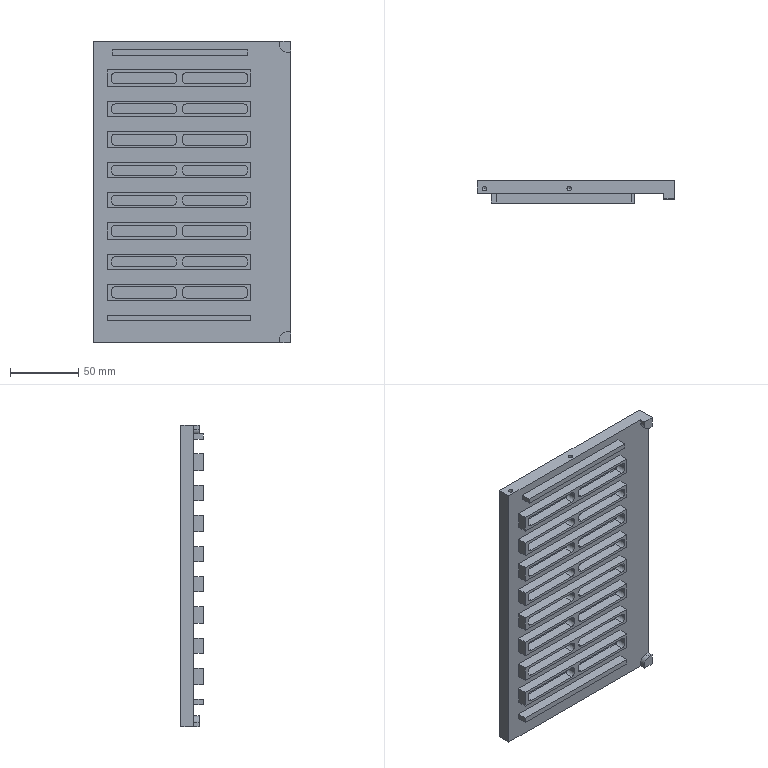NC program | NX | posted with a generic post | part box 144.5 x 16.5 x 221 mm
Lines 3378 to 4181 of 8751:
(动态加工0.5_COPY_1 , TOOL : D5-15-D6-50-3T-ROUGH)
N6748 T03 M6
N6750 G53
N6752 G17 G0 G90 X22.619 Y-60.332 B0. C0. S5000 M3
N6754 G43 Z20. H3
N6756 Z-4.299
N6758 G94 G1 X22.636 Y-60.481 Z-5.236 F1500.
N6760 X22.653 Y-60.63 Z-5.607
N6762 X22.67 Y-60.779 Z-5.879
N6764 X22.686 Y-60.928 Z-6.099
N6766 X22.703 Y-61.077 Z-6.283
N6768 X22.72 Y-61.226 Z-6.441
N6770 X22.737 Y-61.375 Z-6.579
N6772 X22.754 Y-61.524 Z-6.699
N6774 X22.771 Y-61.673 Z-6.804
N6776 X22.787 Y-61.822 Z-6.897
N6778 X22.804 Y-61.971 Z-6.978
N6780 X22.821 Y-62.121 Z-7.049
N6782 X22.838 Y-62.27 Z-7.109
N6784 X22.855 Y-62.419 Z-7.161
N6786 X22.872 Y-62.568 Z-7.204
N6788 X22.888 Y-62.717 Z-7.238
N6790 X22.905 Y-62.866 Z-7.265
N6792 X22.922 Y-63.015 Z-7.284
N6794 X22.939 Y-63.164 Z-7.295
N6796 X22.956 Y-63.313 Z-7.299
N6798 X23.045 Y-64.102
N6800 G3 X23.547 Y-64.55 R0.505
N6802 X25.298 Y-63.147 R2.001
N6804 G1 X25.3 Y-62.787
N6806 G2 X24.701 Y-64.149 R1.509
N6808 X23.619 Y-64.55 R1.349
N6810 G3 X25.295 Y-63.519 R1.549
N6812 G1 X25.3 Y-63.159
N6814 G2 X24.653 Y-64.395 R1.23
N6816 X24.029 Y-64.55 R0.89
N6818 G3 X25.296 Y-63.769 R1.137
N6820 G1 X25.3 Y-63.5
N6822 G2 X24.356 Y-64.55 R0.926
N6824 G3 X25.3 Y-63.914 R0.806
N6826 G1 Y-63.757
N6828 G2 X24.582 Y-64.55 R0.691
N6830 G3 X25.3 Y-63.918 R0.603
N6832 G2 X25.238 Y-64.239 R0.648
N6834 X24.828 Y-64.537 R0.53
N6836 X24.281 Y-64.188 R0.506
N6838 G1 X24.007 Y-63.313
N6840 X23.962 Y-63.17 Z-7.295
N6842 X23.917 Y-63.027 Z-7.284
N6844 X23.872 Y-62.884 Z-7.265
N6846 X23.827 Y-62.741 Z-7.238
N6848 X23.782 Y-62.598 Z-7.204
N6850 X23.737 Y-62.454 Z-7.161
N6852 X23.692 Y-62.311 Z-7.109
N6854 X23.647 Y-62.168 Z-7.049
N6856 X23.602 Y-62.025 Z-6.978
N6858 X23.557 Y-61.882 Z-6.897
N6860 X23.512 Y-61.739 Z-6.804
N6862 X23.467 Y-61.596 Z-6.699
N6864 X23.422 Y-61.453 Z-6.579
N6866 X23.377 Y-61.31 Z-6.441
N6868 X23.332 Y-61.166 Z-6.283
N6870 X23.288 Y-61.023 Z-6.099
N6872 X23.243 Y-60.88 Z-5.879
N6874 X23.198 Y-60.737 Z-5.607
N6876 X23.153 Y-60.594 Z-5.236
N6878 X23.108 Y-60.451 Z-4.299
N6880 G0 Z20.
N6882 X-21.064 Y-62.355
N6884 Z-4.299
N6886 G1 X-21.214 Y-62.353 Z-5.236
N6888 X-21.364 Y-62.35 Z-5.607
N6890 X-21.514 Y-62.347 Z-5.879
N6892 X-21.664 Y-62.345 Z-6.099
N6894 X-21.814 Y-62.342 Z-6.283
N6896 X-21.964 Y-62.34 Z-6.441
N6898 X-22.114 Y-62.337 Z-6.579
N6900 X-22.264 Y-62.335 Z-6.699
N6902 X-22.413 Y-62.332 Z-6.804
N6904 X-22.563 Y-62.33 Z-6.897
N6906 X-22.713 Y-62.327 Z-6.978
N6908 X-22.863 Y-62.324 Z-7.049
N6910 X-23.013 Y-62.322 Z-7.109
N6912 X-23.163 Y-62.319 Z-7.161
N6914 X-23.313 Y-62.317 Z-7.204
N6916 X-23.463 Y-62.314 Z-7.238
N6918 X-23.613 Y-62.312 Z-7.265
N6920 X-23.763 Y-62.309 Z-7.284
N6922 X-23.913 Y-62.307 Z-7.295
N6924 X-24.063 Y-62.304 Z-7.299
N6926 X-24.786 Y-62.292
N6928 G3 X-25.3 Y-62.797 R0.505
N6930 X-23.903 Y-64.548 R2.01
N6932 G1 X-23.541 Y-64.55
N6934 G2 X-24.913 Y-63.935 R1.515
N6936 X-25.3 Y-62.885 R1.328
N6938 G3 X-24.256 Y-64.547 R1.526
N6940 G1 X-23.905 Y-64.55
N6942 G2 X-25.144 Y-63.904 R1.23
N6944 X-25.3 Y-63.278 R0.893
N6946 G3 X-24.532 Y-64.545 R1.143
N6948 G1 X-24.259 Y-64.55
N6950 G2 X-25.3 Y-63.607 R0.924
N6952 G3 X-24.668 Y-64.55 R0.807
N6954 G1 X-24.488
N6956 G2 X-25.3 Y-63.854 R0.694
N6958 G3 X-24.69 Y-64.55 R0.594
N6960 G2 X-24.988 Y-64.488 R0.633
N6962 X-25.287 Y-64.078 R0.53
N6964 X-24.955 Y-63.534 R0.506
N6966 G1 X-24.063 Y-63.221
N6968 X-23.922 Y-63.171 Z-7.295
N6970 X-23.78 Y-63.121 Z-7.284
N6972 X-23.639 Y-63.071 Z-7.265
N6974 X-23.497 Y-63.021 Z-7.238
N6976 X-23.356 Y-62.972 Z-7.204
N6978 X-23.214 Y-62.922 Z-7.161
N6980 X-23.073 Y-62.872 Z-7.109
N6982 X-22.931 Y-62.822 Z-7.049
N6984 X-22.79 Y-62.772 Z-6.978
N6986 X-22.648 Y-62.723 Z-6.897
N6988 X-22.507 Y-62.673 Z-6.804
N6990 X-22.365 Y-62.623 Z-6.699
N6992 X-22.224 Y-62.573 Z-6.579
N6994 X-22.082 Y-62.524 Z-6.441
N6996 X-21.941 Y-62.474 Z-6.283
N6998 X-21.799 Y-62.424 Z-6.099
N7000 X-21.658 Y-62.374 Z-5.879
N7002 X-21.516 Y-62.324 Z-5.607
N7004 X-21.375 Y-62.275 Z-5.236
N7006 X-21.233 Y-62.225 Z-4.299
N7008 G0 Z20.
N7010 X-21.434 Y-61.7
N7012 Z0.3
N7014 G1 X-21.565 Y-61.773 Z-0.637
N7016 X-21.697 Y-61.845 Z-1.008
N7018 X-21.828 Y-61.917 Z-1.28
N7020 X-21.96 Y-61.989 Z-1.5
N7022 X-22.091 Y-62.062 Z-1.684
N7024 X-22.223 Y-62.134 Z-1.842
N7026 X-22.354 Y-62.206 Z-1.98
N7028 X-22.486 Y-62.278 Z-2.1
N7030 X-22.617 Y-62.351 Z-2.205
N7032 X-22.749 Y-62.423 Z-2.298
N7034 X-22.88 Y-62.495 Z-2.379
N7036 X-23.012 Y-62.567 Z-2.45
N7038 X-23.143 Y-62.64 Z-2.51
N7040 X-23.274 Y-62.712 Z-2.562
N7042 X-23.406 Y-62.784 Z-2.605
N7044 X-23.537 Y-62.856 Z-2.639
N7046 X-23.669 Y-62.928 Z-2.666
N7048 X-23.8 Y-63.001 Z-2.685
N7050 X-23.932 Y-63.073 Z-2.696
N7052 X-24.063 Y-63.145 Z-2.7
N7054 X-24.908 Y-63.609
N7056 G3 X-24.845 Y-64.524 R0.505
N7058 X-23.74 Y-64.767 R4.988
N7060 G1 X24.383 Y-64.764
N7062 G3 X25.245 Y-64.348 R1.003
N7064 G1 X25.284 Y-64.243
N7066 G3 X24.637 Y-63.617 R0.519
N7068 G1 X24.364 Y-63.694
N7070 X24.094 Y-63.781
N7072 G3 X24.32 Y-64.767 R0.519
N7074 X25.173 Y-64.536 R1.052
N7076 X25.3 Y-64.178 R0.693
N7078 G2 X24.644 Y-64.767 R0.579
N7080 G3 X24.992 Y-64.703 R0.692
N7082 X25.237 Y-64.457 R0.561
N7084 X25.076 Y-63.864 R0.501
N7086 G1 X24.869 Y-63.709
N7088 X24.486 Y-63.417 Z-2.603
N7090 X24.095 Y-63.137 Z-2.505
N7092 X24.071 Y-63.125 Z-2.5
N7094 X23.967 Y-63.093 F15000.
N7096 X23.86 Y-63.08
N7098 X-22.363 Y-63.39
N7100 G3 X-22.698 Y-63.521 R0.509
N7102 G1 X-22.818 Y-63.679 Z-2.54 F1500.
N7104 X-22.916 Y-63.85 Z-2.58
N7106 X-23.216 Y-64.362 Z-2.7
N7108 X-23.306 Y-64.516
N7110 X-23.421 Y-64.652
N7112 G2 X-23.74 Y-64.767 R0.511
N7114 X-25.032 Y-64.527 R2.277
N7116 X-25.25 Y-64.288 R0.996
N7118 X-24.624 Y-63.524 R0.55
N7120 G1 X-24.244 Y-63.611
N7122 X-23.868 Y-63.709
N7124 G2 X-24.078 Y-64.767 R0.55
N7126 X-25.147 Y-64.489 R1.427
N7128 X-25.287 Y-64.236 R1.13
N7130 X-24.597 Y-63.63 R0.522
N7132 G1 X-24.179 Y-63.792
N7134 G2 X-24.438 Y-64.767 R0.522
N7136 X-25.293 Y-64.257 R0.747
N7138 G1 X-25.3 Y-64.178
N7140 G3 X-24.599 Y-64.767 R0.59
N7142 G2 X-25.031 Y-64.687 R0.792
N7144 X-25.237 Y-64.457 R0.524
N7146 X-24.917 Y-63.779 R0.505
N7148 G1 X-24.063 Y-63.521
N7150 X-23.92 Y-63.477 Z-2.696
N7152 X-23.776 Y-63.434 Z-2.685
N7154 X-23.633 Y-63.39 Z-2.666
N7156 X-23.489 Y-63.347 Z-2.639
N7158 X-23.345 Y-63.304 Z-2.605
N7160 X-23.202 Y-63.26 Z-2.562
N7162 X-23.058 Y-63.217 Z-2.51
N7164 X-22.915 Y-63.173 Z-2.45
N7166 X-22.771 Y-63.13 Z-2.379
N7168 X-22.627 Y-63.087 Z-2.298
N7170 X-22.484 Y-63.043 Z-2.205
N7172 X-22.34 Y-63. Z-2.1
N7174 X-22.197 Y-62.956 Z-1.98
N7176 X-22.053 Y-62.913 Z-1.842
N7178 X-21.91 Y-62.87 Z-1.684
N7180 X-21.766 Y-62.826 Z-1.5
N7182 X-21.622 Y-62.783 Z-1.28
N7184 X-21.479 Y-62.739 Z-1.008
N7186 X-21.335 Y-62.696 Z-0.637
N7188 X-21.192 Y-62.652 Z0.3
N7190 G0 Z20.
N7192 X-21.369 Y-62.09
N7194 Z0.6
N7196 G1 X-21.504 Y-62.156 Z-0.337
N7198 X-21.639 Y-62.222 Z-0.708
N7200 X-21.773 Y-62.288 Z-0.98
N7202 X-21.908 Y-62.354 Z-1.2
N7204 X-22.043 Y-62.42 Z-1.384
N7206 X-22.177 Y-62.486 Z-1.542
N7208 X-22.312 Y-62.552 Z-1.68
N7210 X-22.447 Y-62.618 Z-1.8
N7212 X-22.582 Y-62.684 Z-1.905
N7214 X-22.716 Y-62.75 Z-1.998
N7216 X-22.851 Y-62.816 Z-2.079
N7218 X-22.986 Y-62.882 Z-2.15
N7220 X-23.12 Y-62.948 Z-2.21
N7222 X-23.255 Y-63.014 Z-2.262
N7224 X-23.39 Y-63.08 Z-2.305
N7226 X-23.524 Y-63.146 Z-2.339
N7228 X-23.659 Y-63.212 Z-2.366
N7230 X-23.794 Y-63.278 Z-2.385
N7232 X-23.929 Y-63.344 Z-2.396
N7234 X-24.063 Y-63.41 Z-2.4
N7236 X-24.889 Y-63.814
N7238 G3 X-24.844 Y-64.741 R0.505
N7240 X-23.028 Y-65.012 R5.818
N7242 X-16.678 Y-65.067 R217.96
N7244 G1 X23.727 Y-65.066
N7246 G3 X24.988 Y-64.831 R2.542
N7248 X25.291 Y-64.439 R0.61
N7250 X24.966 Y-63.872 R0.505
N7252 G1 X24.068 Y-63.458 Z-2.2
N7254 G2 X23.751 Y-62.741 R0.528 F15000.
N7256 X24.046 Y-62.457 R0.505
N7258 X24.696 Y-62.783 Z-2.364 R0.506 F1500.
N7260 G1 X24.761 Y-62.948 Z-2.4
N7262 X25.284 Y-64.273
N7264 G2 X24.895 Y-64.928 R0.596
N7266 X24.473 Y-65.067 R3.243
N7268 G1 X-23.726 Y-65.065
N7270 G2 X-25.045 Y-64.74 R2.603
N7272 X-25.263 Y-64.478 R0.828
N7274 X-24.67 Y-63.789 R0.513
N7276 G1 X-23.537 Y-64.056
N7278 G2 X-23.654 Y-65.067 R0.513
N7280 X-24.847 Y-64.922 R2.743
N7282 X-25.29 Y-64.45 R0.725
N7284 X-24.592 Y-63.826 R0.55
N7286 G1 X-24.273 Y-63.918
N7288 X-23.957 Y-64.021
N7290 G2 X-24.194 Y-65.067 R0.55
N7292 X-25.249 Y-64.63 R1.075
N7294 G1 X-25.295 Y-64.48
N7296 G2 X-24.563 Y-63.897 R0.55
N7298 G1 X-24.196 Y-64.037
N7300 G2 X-24.464 Y-65.067 R0.55
N7302 X-25.297 Y-64.515 R0.739
N7304 X-24.546 Y-63.951 R0.547
N7306 G1 X-24.387 Y-64.016
N7308 X-24.242 Y-64.106
N7310 G2 X-24.599 Y-65.067 R0.547
N7312 X-25.3 Y-64.388 R0.626
N7314 G3 X-24.689 Y-65.067 R0.584
N7316 X-24.257 Y-64.819 R0.502
N7318 G1 X-24.172 Y-64.673
N7320 X-23.704 Y-63.881 Z-2.214
N7322 X-23.658 Y-63.83 Z-2.2
N7324 G2 X-23.311 Y-63.69 R0.508 F15000.
N7326 G1 X23.096
N7328 G2 X23.435 Y-63.822 R0.509
N7330 G1 X23.555 Y-63.98 Z-2.24 F1500.
N7332 X23.652 Y-64.152 Z-2.28
N7334 X23.951 Y-64.664 Z-2.4
N7336 X24.039 Y-64.816
N7338 X24.153 Y-64.951
N7340 G3 X24.473 Y-65.067 R0.511
N7342 X25.293 Y-64.555 R0.731
N7344 G1 X25.3 Y-64.388
N7346 G2 X24.599 Y-65.067 R0.617
N7348 G3 X25.288 Y-64.592 R0.59
N7350 X24.948 Y-64.047 R0.506
N7352 G1 X24.063 Y-63.75
N7354 X23.921 Y-63.703 Z-2.396
N7356 X23.779 Y-63.655 Z-2.385
N7358 X23.637 Y-63.607 Z-2.366
N7360 X23.494 Y-63.56 Z-2.339
N7362 X23.352 Y-63.512 Z-2.305
N7364 X23.21 Y-63.464 Z-2.262
N7366 X23.068 Y-63.417 Z-2.21
N7368 X22.925 Y-63.369 Z-2.15
N7370 X22.783 Y-63.322 Z-2.079
N7372 X22.641 Y-63.274 Z-1.998
N7374 X22.499 Y-63.226 Z-1.905
N7376 X22.357 Y-63.179 Z-1.8
N7378 X22.214 Y-63.131 Z-1.68
N7380 X22.072 Y-63.083 Z-1.542
N7382 X21.93 Y-63.036 Z-1.384
N7384 X21.788 Y-62.988 Z-1.2
N7386 X21.645 Y-62.94 Z-0.98
N7388 X21.503 Y-62.893 Z-0.708
N7390 X21.361 Y-62.845 Z-0.337
N7392 X21.219 Y-62.797 Z0.6
N7394 G0 Z20.
N7396 X-21.361 Y-62.413
N7398 Z0.9
N7400 G1 X-21.496 Y-62.478 Z-0.037
N7402 X-21.631 Y-62.543 Z-0.408
N7404 X-21.766 Y-62.608 Z-0.68
N7406 X-21.902 Y-62.673 Z-0.9
N7408 X-22.037 Y-62.739 Z-1.084
N7410 X-22.172 Y-62.804 Z-1.242
N7412 X-22.307 Y-62.869 Z-1.38
N7414 X-22.442 Y-62.934 Z-1.5
N7416 X-22.577 Y-62.999 Z-1.605
N7418 X-22.712 Y-63.064 Z-1.698
N7420 X-22.847 Y-63.13 Z-1.779
N7422 X-22.982 Y-63.195 Z-1.85
N7424 X-23.118 Y-63.26 Z-1.91
N7426 X-23.253 Y-63.325 Z-1.962
N7428 X-23.388 Y-63.39 Z-2.005
N7430 X-23.523 Y-63.455 Z-2.039
N7432 X-23.658 Y-63.521 Z-2.066
N7434 X-23.793 Y-63.586 Z-2.085
N7436 X-23.928 Y-63.651 Z-2.096
N7438 X-24.063 Y-63.716 Z-2.1
N7440 X-24.886 Y-64.113
N7442 G3 X-24.844 Y-65.041 R0.505
N7444 X-22.946 Y-65.316 R6.069
N7446 X-16.565 Y-65.367 R250.064
N7448 G1 X23.727 Y-65.366
N7450 G3 X25.009 Y-65.118 R2.474
N7452 X25.289 Y-64.751 R0.607
N7454 X24.966 Y-64.183 R0.505
N7456 G1 X24.068 Y-63.768 Z-1.9
N7458 G2 X23.726 Y-63.122 R0.522 F15000.
N7460 X24.046 Y-62.755 R0.502
N7462 X24.696 Y-63.082 Z-2.064 R0.505 F1500.
N7464 G1 X24.761 Y-63.246 Z-2.1
N7466 X25.284 Y-64.573
N7468 G2 X24.881 Y-65.235 R0.602
N7470 X24.472 Y-65.367 R3.661
N7472 G1 X-23.731 Y-65.365
N7474 G2 X-25.008 Y-65.066 R2.764
N7476 X-25.255 Y-64.8 R0.847
N7478 X-24.634 Y-64.051 R0.55
N7480 G1 X-23.543 Y-64.279
N7482 G2 X-23.655 Y-65.367 R0.55
N7484 X-24.874 Y-65.209 R2.663
N7486 X-25.29 Y-64.748 R0.708
N7488 X-24.592 Y-64.126 R0.55
N7490 G1 X-24.273 Y-64.218
N7492 X-23.958 Y-64.321
N7494 G2 X-24.195 Y-65.367 R0.55
N7496 X-25.241 Y-64.947 R1.087
N7498 G1 X-25.295 Y-64.776
N7500 G2 X-24.569 Y-64.205 R0.538
N7502 G1 X-24.17 Y-64.366
N7504 G2 X-24.443 Y-65.367 R0.538
N7506 X-25.297 Y-64.814 R0.748
N7508 X-24.545 Y-64.252 R0.547
N7510 G1 X-24.387 Y-64.316
N7512 X-24.242 Y-64.407
N7514 G2 X-24.6 Y-65.367 R0.547
N7516 X-25.3 Y-64.688 R0.626
N7518 G3 X-24.688 Y-65.367 R0.585
N7520 X-24.256 Y-65.119 R0.502
N7522 G1 X-24.172 Y-64.973
N7524 X-23.704 Y-64.181 Z-1.914
N7526 X-23.658 Y-64.13 Z-1.9
N7528 G2 X-23.311 Y-63.99 R0.508 F15000.
N7530 G1 X23.095
N7532 G2 X23.434 Y-64.122 R0.509
N7534 G1 X23.554 Y-64.28 Z-1.94 F1500.
N7536 X23.651 Y-64.452 Z-1.98
N7538 X23.95 Y-64.964 Z-2.1
N7540 X24.039 Y-65.116
N7542 X24.152 Y-65.251
N7544 G3 X24.472 Y-65.367 R0.511
N7546 X25.293 Y-64.855 R0.732
N7548 G1 X25.3 Y-64.688
N7550 G2 X24.598 Y-65.367 R0.617
N7552 G3 X25.288 Y-64.892 R0.59
N7554 X24.944 Y-64.345 R0.506
N7556 G1 X24.063 Y-64.058
N7558 X23.921 Y-64.012 Z-2.096
N7560 X23.778 Y-63.965 Z-2.085
N7562 X23.635 Y-63.919 Z-2.066
N7564 X23.493 Y-63.872 Z-2.039
N7566 X23.35 Y-63.826 Z-2.005
N7568 X23.208 Y-63.779 Z-1.962
N7570 X23.065 Y-63.733 Z-1.91
N7572 X22.922 Y-63.686 Z-1.85
N7574 X22.78 Y-63.64 Z-1.779
N7576 X22.637 Y-63.594 Z-1.698
N7578 X22.494 Y-63.547 Z-1.605
N7580 X22.352 Y-63.501 Z-1.5
N7582 X22.209 Y-63.454 Z-1.38
N7584 X22.067 Y-63.408 Z-1.242
N7586 X21.924 Y-63.361 Z-1.084
N7588 X21.781 Y-63.315 Z-0.9
N7590 X21.639 Y-63.268 Z-0.68
N7592 X21.496 Y-63.222 Z-0.408
N7594 X21.354 Y-63.175 Z-0.037
N7596 X21.211 Y-63.129 Z0.9
N7598 G0 Z20.
N7600 X-21.358 Y-62.722
N7602 Z1.2
N7604 G1 X-21.493 Y-62.787 Z0.263
N7606 X-21.629 Y-62.851 Z-0.108
N7608 X-21.764 Y-62.916 Z-0.38
N7610 X-21.899 Y-62.981 Z-0.6
N7612 X-22.034 Y-63.046 Z-0.784
N7614 X-22.17 Y-63.111 Z-0.942
N7616 X-22.305 Y-63.176 Z-1.08
N7618 X-22.44 Y-63.24 Z-1.2
N7620 X-22.575 Y-63.305 Z-1.305
N7622 X-22.711 Y-63.37 Z-1.398
N7624 X-22.846 Y-63.435 Z-1.479
N7626 X-22.981 Y-63.5 Z-1.55
N7628 X-23.116 Y-63.565 Z-1.61
N7630 X-23.252 Y-63.629 Z-1.662
N7632 X-23.387 Y-63.694 Z-1.705
N7634 X-23.522 Y-63.759 Z-1.739
N7636 X-23.657 Y-63.824 Z-1.766
N7638 X-23.793 Y-63.889 Z-1.785
N7640 X-23.928 Y-63.954 Z-1.796
N7642 X-24.063 Y-64.018 Z-1.8
N7644 X-24.885 Y-64.413
N7646 G3 X-24.844 Y-65.341 R0.505
N7648 X-23.616 Y-65.667 R7.48
N7650 G1 X23.993 Y-65.662
N7652 G3 X25.167 Y-65.29 R1.708
N7654 X25.288 Y-65.052 R2.064
N7656 X24.643 Y-64.408 R0.55
N7658 G1 X24.165 Y-64.498
N7660 X23.689 Y-64.602
N7662 G3 X23.881 Y-65.667 R0.55
N7664 X24.87 Y-65.586 R2.717
N7666 X25.297 Y-65.102 R0.626
N7668 X24.588 Y-64.522 R0.547
N7670 G1 X24.262 Y-64.634
N7672 G3 X24.511 Y-65.667 R0.547
N7674 X25.282 Y-65.236 R0.671
N7676 G1 X25.3 Y-64.988
N7678 G2 X25.245 Y-65.338 R0.727
N7680 X24.711 Y-65.667 R0.557
N7682 G3 X25.22 Y-65.398 R0.587
N7684 G1 X25.228 Y-65.378
N7686 G3 X25.067 Y-64.785 R0.501
N7688 G1 X24.868 Y-64.636
N7690 X24.114 Y-64.073 Z-1.61
N7692 X24.071 Y-64.05 Z-1.6
N7694 X23.964 Y-64.014 F15000.
N7696 X23.851 Y-64.
N7698 X-22.239 Y-64.29
N7700 G3 X-22.574 Y-64.421 R0.509
N7702 G1 X-22.694 Y-64.579 Z-1.64 F1500.
N7704 X-22.792 Y-64.75 Z-1.68
N7706 X-23.092 Y-65.262 Z-1.8
N7708 X-23.182 Y-65.416
N7710 X-23.297 Y-65.552
N7712 G2 X-23.616 Y-65.667 R0.511
N7714 X-25.057 Y-65.333 R2.545
N7716 X-25.262 Y-65.083 R0.929
N7718 X-24.649 Y-64.395 R0.513
N7720 G1 X-24.133 Y-64.536
N7722 X-23.622 Y-64.692
N7724 G2 X-23.841 Y-65.667 R0.513
N7726 X-25.084 Y-65.375 R1.829
N7728 X-25.293 Y-65.031 R0.643
N7730 X-24.595 Y-64.445 R0.531
N7732 G1 X-24.28 Y-64.551
N7734 X-23.969 Y-64.669
N7736 G2 X-24.224 Y-65.667 R0.531
N7738 X-25.258 Y-65.209 R1.023
N7740 G1 X-25.298 Y-65.058
N7742 G2 X-24.551 Y-64.496 R0.55
N7744 G1 X-24.192 Y-64.644
N7746 G2 X-24.471 Y-65.667 R0.55
N7748 X-25.297 Y-65.116 R0.736
N7750 X-24.539 Y-64.555 R0.547
N7752 X-24.182 Y-64.775 R0.832
N7754 X-24.606 Y-65.667 R0.547
N7756 X-25.3 Y-64.988 R0.625
N7758 G3 X-24.688 Y-65.667 R0.585
N7760 X-24.205 Y-65.307 R0.506
N7762 G1 X-23.942 Y-64.43
N7764 X-23.899 Y-64.287 Z-1.796
N7766 X-23.856 Y-64.143 Z-1.785
N7768 X-23.813 Y-63.999 Z-1.766
N7770 X-23.77 Y-63.856 Z-1.739
N7772 X-23.727 Y-63.712 Z-1.705
N7774 X-23.684 Y-63.568 Z-1.662
N7776 X-23.641 Y-63.425 Z-1.61
N7778 X-23.597 Y-63.281 Z-1.55
N7780 X-23.554 Y-63.137 Z-1.479
N7782 X-23.511 Y-62.994 Z-1.398
N7784 X-23.468 Y-62.85 Z-1.305
N7786 X-23.425 Y-62.706 Z-1.2
N7788 X-23.382 Y-62.562 Z-1.08
N7790 X-23.339 Y-62.419 Z-0.942
N7792 X-23.296 Y-62.275 Z-0.784
N7794 X-23.253 Y-62.131 Z-0.6
N7796 X-23.21 Y-61.988 Z-0.38
N7798 X-23.167 Y-61.844 Z-0.108
N7800 X-23.124 Y-61.7 Z0.263
N7802 X-23.081 Y-61.557 Z1.2
N7804 G0 Z20.
N7806 X-21.358 Y-63.022
N7808 Z1.5
N7810 G1 X-21.493 Y-63.087 Z0.563
N7812 X-21.629 Y-63.151 Z0.192
N7814 X-21.764 Y-63.216 Z-0.08
N7816 X-21.899 Y-63.281 Z-0.3
N7818 X-22.034 Y-63.346 Z-0.484
N7820 X-22.17 Y-63.411 Z-0.642
N7822 X-22.305 Y-63.476 Z-0.78
N7824 X-22.44 Y-63.54 Z-0.9
N7826 X-22.575 Y-63.605 Z-1.005
N7828 X-22.711 Y-63.67 Z-1.098
N7830 X-22.846 Y-63.735 Z-1.179
N7832 X-22.981 Y-63.8 Z-1.25
N7834 X-23.116 Y-63.865 Z-1.31
N7836 X-23.252 Y-63.929 Z-1.362
N7838 X-23.387 Y-63.994 Z-1.405
N7840 X-23.522 Y-64.059 Z-1.439
N7842 X-23.657 Y-64.124 Z-1.466
N7844 X-23.793 Y-64.189 Z-1.485
N7846 X-23.928 Y-64.254 Z-1.496
N7848 X-24.063 Y-64.319 Z-1.5
N7850 X-24.885 Y-64.713
N7852 G3 X-24.844 Y-65.641 R0.505
N7854 X-22.946 Y-65.916 R6.068
N7856 X-16.565 Y-65.967 R249.964
N7858 G1 X23.727 Y-65.966
N7860 G3 X25.009 Y-65.718 R2.475
N7862 X25.289 Y-65.351 R0.607
N7864 X24.966 Y-64.783 R0.505
N7866 G1 X24.068 Y-64.368 Z-1.3
N7868 G2 X23.726 Y-63.722 R0.522 F15000.
N7870 X24.046 Y-63.355 R0.502
N7872 X24.696 Y-63.682 Z-1.464 R0.505 F1500.
N7874 G1 X24.761 Y-63.846 Z-1.5
N7876 X25.284 Y-65.173
N7878 G2 X24.881 Y-65.835 R0.602
N7880 X24.472 Y-65.967 R3.658
N7882 G1 X-23.731 Y-65.965
N7884 G2 X-25.008 Y-65.666 R2.764
N7886 X-25.255 Y-65.4 R0.847
N7888 X-24.634 Y-64.651 R0.55
N7890 G1 X-23.543 Y-64.879
N7892 G2 X-23.656 Y-65.967 R0.55
N7894 X-24.874 Y-65.809 R2.662
N7896 X-25.29 Y-65.348 R0.708
N7898 X-24.592 Y-64.726 R0.55
N7900 G1 X-24.273 Y-64.818
N7902 X-23.958 Y-64.921
N7904 G2 X-24.196 Y-65.967 R0.55
N7906 X-25.241 Y-65.547 R1.086
N7908 G1 X-25.295 Y-65.376
N7910 G2 X-24.569 Y-64.805 R0.538
N7912 G1 X-24.171 Y-64.966
N7914 G2 X-24.443 Y-65.967 R0.538
N7916 X-25.297 Y-65.414 R0.748
N7918 X-24.545 Y-64.852 R0.547
N7920 G1 X-24.387 Y-64.916
N7922 X-24.242 Y-65.007
N7924 G2 X-24.601 Y-65.967 R0.547
N7926 X-25.3 Y-65.288 R0.627
N7928 G3 X-24.688 Y-65.967 R0.585
N7930 X-24.256 Y-65.719 R0.502
N7932 G1 X-24.171 Y-65.573
N7934 X-23.704 Y-64.781 Z-1.314
N7936 X-23.658 Y-64.73 Z-1.3
N7938 G2 X-23.311 Y-64.59 R0.508 F15000.
N7940 G1 X23.095
N7942 G2 X23.434 Y-64.722 R0.509
N7944 G1 X23.553 Y-64.88 Z-1.34 F1500.
N7946 X23.651 Y-65.052 Z-1.38
N7948 X23.95 Y-65.564 Z-1.5
N7950 X24.038 Y-65.716
N7952 X24.152 Y-65.851
N7954 G3 X24.472 Y-65.967 R0.511
N7956 X25.293 Y-65.455 R0.732
N7958 G1 X25.3 Y-65.288
N7960 G2 X24.598 Y-65.967 R0.618
N7962 G3 X25.288 Y-65.492 R0.59
N7964 X24.942 Y-64.944 R0.506
N7966 G1 X24.063 Y-64.661
N7968 X23.921 Y-64.615 Z-1.496
N7970 X23.778 Y-64.569 Z-1.485
N7972 X23.635 Y-64.523 Z-1.466
N7974 X23.492 Y-64.477 Z-1.439
N7976 X23.349 Y-64.431 Z-1.405
N7978 X23.207 Y-64.385 Z-1.362
N7980 X23.064 Y-64.339 Z-1.31
N7982 X22.921 Y-64.293 Z-1.25
N7984 X22.778 Y-64.247 Z-1.179
N7986 X22.636 Y-64.201 Z-1.098
N7988 X22.493 Y-64.155 Z-1.005
N7990 X22.35 Y-64.109 Z-0.9
N7992 X22.207 Y-64.063 Z-0.78
N7994 X22.064 Y-64.017 Z-0.642
N7996 X21.922 Y-63.971 Z-0.484
N7998 X21.779 Y-63.925 Z-0.3
N8000 X21.636 Y-63.879 Z-0.08
N8002 X21.493 Y-63.833 Z0.192
N8004 X21.351 Y-63.787 Z0.563
N8006 X21.208 Y-63.741 Z1.5
N8008 G0 Z20.
N8010 X-21.358 Y-63.322
N8012 Z1.8
N8014 G1 X-21.493 Y-63.387 Z0.863
N8016 X-21.629 Y-63.451 Z0.492
N8018 X-21.764 Y-63.516 Z0.22
N8020 X-21.899 Y-63.581 Z0.
N8022 X-22.034 Y-63.646 Z-0.184
N8024 X-22.17 Y-63.711 Z-0.342
N8026 X-22.305 Y-63.776 Z-0.48
N8028 X-22.44 Y-63.84 Z-0.6
N8030 X-22.575 Y-63.905 Z-0.705
N8032 X-22.711 Y-63.97 Z-0.798
N8034 X-22.846 Y-64.035 Z-0.879
N8036 X-22.981 Y-64.1 Z-0.95
N8038 X-23.116 Y-64.165 Z-1.01
N8040 X-23.252 Y-64.229 Z-1.062
N8042 X-23.387 Y-64.294 Z-1.105
N8044 X-23.522 Y-64.359 Z-1.139
N8046 X-23.657 Y-64.424 Z-1.166
N8048 X-23.793 Y-64.489 Z-1.185
N8050 X-23.928 Y-64.554 Z-1.196
N8052 X-24.063 Y-64.619 Z-1.2
N8054 X-24.885 Y-65.012
N8056 G3 X-24.844 Y-65.941 R0.505
N8058 X-22.946 Y-66.216 R6.067
N8060 X-16.565 Y-66.267 R249.933
N8062 G1 X23.67 Y-66.266
N8064 G3 X24.956 Y-66.051 R2.782
N8066 X25.289 Y-65.651 R0.636
N8068 X24.966 Y-65.083 R0.505
N8070 G1 X24.068 Y-64.668 Z-1.
N8072 G2 X23.726 Y-64.022 R0.522 F15000.
N8074 X24.046 Y-63.655 R0.502
N8076 X24.696 Y-63.982 Z-1.164 R0.505 F1500.
N8078 G1 X24.761 Y-64.146 Z-1.2
N8080 X25.284 Y-65.473
N8082 G2 X24.881 Y-66.135 R0.602
N8084 X24.472 Y-66.267 R3.651
N8086 G1 X-23.731 Y-66.265
N8088 G2 X-25.008 Y-65.966 R2.765
N8090 X-25.255 Y-65.699 R0.847
N8092 X-24.634 Y-64.951 R0.55
N8094 G1 X-23.543 Y-65.179
N8096 G2 X-23.656 Y-66.267 R0.55
N8098 X-24.874 Y-66.109 R2.662
N8100 X-25.29 Y-65.648 R0.708
N8102 X-24.592 Y-65.026 R0.55
N8104 G1 X-24.273 Y-65.118
N8106 X-23.958 Y-65.221
N8108 G2 X-24.196 Y-66.267 R0.55
N8110 X-25.241 Y-65.847 R1.086
N8112 G1 X-25.295 Y-65.676
N8114 G2 X-24.569 Y-65.105 R0.538
N8116 G1 X-24.171 Y-65.266
N8118 G2 X-24.443 Y-66.267 R0.538
N8120 X-25.297 Y-65.714 R0.748
N8122 X-24.545 Y-65.152 R0.547
N8124 G1 X-24.387 Y-65.216
N8126 X-24.242 Y-65.307
N8128 G2 X-24.601 Y-66.267 R0.547
N8130 X-25.3 Y-65.588 R0.627
N8132 G3 X-24.688 Y-66.267 R0.585
N8134 X-24.256 Y-66.019 R0.502
N8136 G1 X-24.171 Y-65.873
N8138 X-23.704 Y-65.081 Z-1.014
N8140 X-23.658 Y-65.03 Z-1.
N8142 G2 X-23.311 Y-64.89 R0.508 F15000.
N8144 G1 X23.095
N8146 G2 X23.434 Y-65.022 R0.509
N8148 G1 X23.553 Y-65.18 Z-1.04 F1500.
N8150 X23.651 Y-65.352 Z-1.08
N8152 X23.95 Y-65.864 Z-1.2
N8154 X24.038 Y-66.016
N8156 X24.152 Y-66.151
N8158 G3 X24.472 Y-66.267 R0.511
N8160 X25.293 Y-65.755 R0.732
N8162 G1 X25.3 Y-65.588
N8164 G2 X24.598 Y-66.267 R0.618
N8166 G3 X25.288 Y-65.791 R0.59
N8168 X24.943 Y-65.247 R0.506
N8170 G1 X24.063 Y-64.961
N8172 X23.921 Y-64.915 Z-1.196
N8174 X23.778 Y-64.868 Z-1.185
N8176 X23.635 Y-64.822 Z-1.166
N8178 X23.493 Y-64.775 Z-1.139
N8180 X23.35 Y-64.729 Z-1.105
N8182 X23.207 Y-64.683 Z-1.062
N8184 X23.065 Y-64.636 Z-1.01
N8186 X22.922 Y-64.59 Z-0.95
N8188 X22.779 Y-64.544 Z-0.879
N8190 X22.637 Y-64.497 Z-0.798
N8192 X22.494 Y-64.451 Z-0.705
N8194 X22.351 Y-64.404 Z-0.6
N8196 X22.209 Y-64.358 Z-0.48
N8198 X22.066 Y-64.312 Z-0.342
N8200 X21.923 Y-64.265 Z-0.184
N8202 X21.781 Y-64.219 Z0.
N8204 X21.638 Y-64.173 Z0.22
N8206 X21.496 Y-64.126 Z0.492
N8208 X21.353 Y-64.08 Z0.863
N8210 X21.21 Y-64.034 Z1.8
N8212 G0 Z20.
N8214 X-21.333 Y-63.671
N8216 Z2.1
N8218 G1 X-21.47 Y-63.733 Z1.163
N8220 X-21.606 Y-63.796 Z0.792
N8222 X-21.743 Y-63.858 Z0.52
N8224 X-21.879 Y-63.92 Z0.3
N8226 X-22.016 Y-63.982 Z0.116
N8228 X-22.152 Y-64.044 Z-0.042
N8230 X-22.289 Y-64.106 Z-0.18
N8232 X-22.425 Y-64.169 Z-0.3
N8234 X-22.562 Y-64.231 Z-0.405
N8236 X-22.698 Y-64.293 Z-0.498
N8238 X-22.835 Y-64.355 Z-0.579
N8240 X-22.971 Y-64.417 Z-0.65
N8242 X-23.108 Y-64.48 Z-0.71
N8244 X-23.244 Y-64.542 Z-0.762
N8246 X-23.381 Y-64.604 Z-0.805
N8248 X-23.517 Y-64.666 Z-0.839
N8250 X-23.654 Y-64.728 Z-0.866
N8252 X-23.79 Y-64.79 Z-0.885
N8254 X-23.927 Y-64.853 Z-0.896
N8256 X-24.063 Y-64.915 Z-0.9
N8258 X-24.883 Y-65.288
N8260 G3 X-24.832 Y-66.228 R0.505
N8262 X-23.867 Y-66.567 R5.725
N8264 G1 X23.993 Y-66.562
N8266 G3 X25.168 Y-66.19 R1.707
N8268 X25.288 Y-65.952 R2.064
N8270 X24.643 Y-65.308 R0.55
N8272 G1 X24.163 Y-65.398
N8274 X23.687 Y-65.502
N8276 G3 X23.878 Y-66.567 R0.55
N8278 X24.87 Y-66.486 R2.729
N8280 X25.297 Y-66.002 R0.626
N8282 X24.59 Y-65.422 R0.547
N8284 G1 X24.265 Y-65.531
N8286 G3 X24.508 Y-66.567 R0.547
N8288 X25.282 Y-66.136 R0.673
N8290 G1 X25.3 Y-65.888
N8292 G2 X25.245 Y-66.238 R0.728
N8294 X24.71 Y-66.567 R0.557
N8296 G3 X25.22 Y-66.298 R0.588
N8298 G1 X25.229 Y-66.277
N8300 G3 X25.067 Y-65.685 R0.501
N8302 G1 X24.868 Y-65.535
N8304 X24.114 Y-64.973 Z-0.71
N8306 X24.071 Y-64.949 Z-0.7
N8308 X23.964 Y-64.914 F15000.
N8310 X23.851 Y-64.9
N8312 X-22.489 Y-65.19
N8314 G3 X-22.824 Y-65.322 R0.509
N8316 G1 X-22.944 Y-65.479 Z-0.74 F1500.
N8318 X-23.042 Y-65.65 Z-0.78
N8320 X-23.343 Y-66.162 Z-0.9
N8322 X-23.432 Y-66.316
N8324 X-23.547 Y-66.452
N8326 G2 X-23.867 Y-66.567 R0.511
N8328 X-25.132 Y-66.17 R2.109
N8330 G1 X-25.26 Y-65.987
N8332 G2 X-24.594 Y-65.259 R0.55
N8334 G1 X-24.156 Y-65.383
N8336 X-23.721 Y-65.52
N8338 G2 X-23.957 Y-66.567 R0.55
N8340 X-25.203 Y-66.153 R1.469
N8342 G1 X-25.295 Y-65.925
N8344 G2 X-24.594 Y-65.344 R0.534
N8346 G1 X-24.282 Y-65.447
N8348 X-23.974 Y-65.562